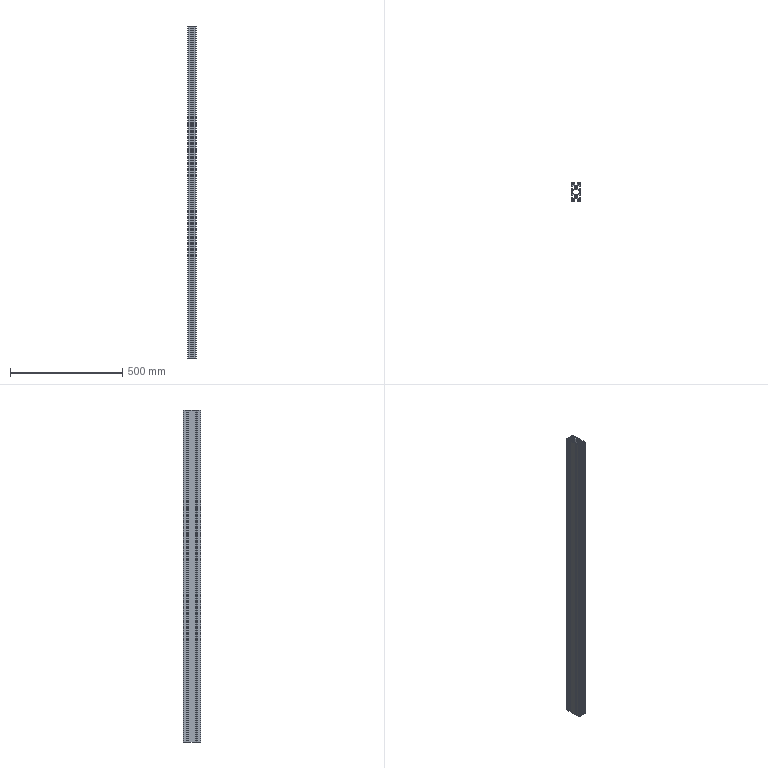Part | NX | features BREP 1 | 1 solid | 182 faces | box 40 x 80 x 1476 mm | volume 1644635 mm3 | plane 112 | cylinder 70 | commonest cylinder face diameters 2 x36 0.76 x20 10.5 x10 6 x4